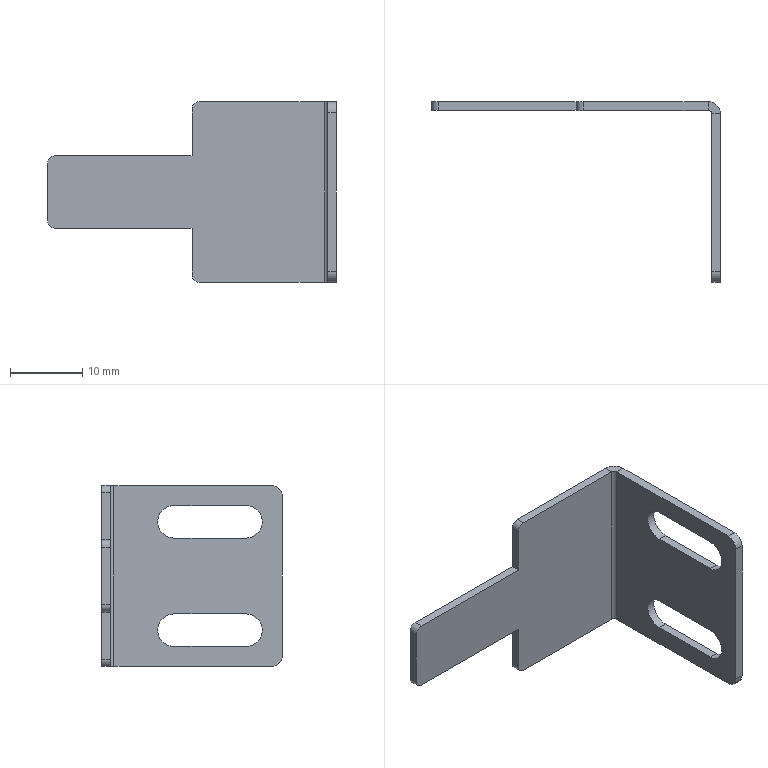Part | SolidWorks | features Fillet 2, FlatPattern 1, HoleWzd 1, ICE 1, SMBaseFlange 1, SheetMetal 1 | 1 solid | 32 faces | box 40 x 25 x 25 mm | volume 1391 mm3 | plane 20 | cylinder 12 | commonest cylinder face diameters 2 x4 4.5 x4 3 x2 1 x1 3.4 x1
STEP:
#1=CARTESIAN_POINT('',(0.,-10.,-5.25));
#2=VERTEX_POINT('',#1);
#3=CARTESIAN_POINT('',(0.,-10.,-9.75));
#4=VERTEX_POINT('',#3);
#5=CARTESIAN_POINT('',(0.,-10.,-7.5));
#6=DIRECTION('',(-1.,0.,0.));
#7=DIRECTION('',(0.,0.,1.));
#8=AXIS2_PLACEMENT_3D('',#5,#6,#7);
#9=CIRCLE('',#8,2.25);
#10=EDGE_CURVE('',#2,#4,#9,.T.);
#11=ORIENTED_EDGE('',*,*,#10,.T.);
#12=CARTESIAN_POINT('',(0.,-20.,-9.75));
#13=VERTEX_POINT('',#12);
#14=CARTESIAN_POINT('',(0.,-20.,-9.75));
#15=DIRECTION('',(0.,1.,0.));
#16=VECTOR('',#15,1000.);
#17=LINE('',#14,#16);
#18=EDGE_CURVE('',#13,#4,#17,.T.);
#19=ORIENTED_EDGE('',*,*,#18,.F.);
#20=CARTESIAN_POINT('',(0.,-20.,-5.25));
#21=VERTEX_POINT('',#20);
#22=CARTESIAN_POINT('',(0.,-20.,-7.5));
#23=DIRECTION('',(-1.,0.,0.));
#24=DIRECTION('',(0.,0.,1.));
#25=AXIS2_PLACEMENT_3D('',#22,#23,#24);
#26=CIRCLE('',#25,2.25);
#27=EDGE_CURVE('',#13,#21,#26,.T.);
#28=ORIENTED_EDGE('',*,*,#27,.T.);
#29=CARTESIAN_POINT('',(0.,-20.,-5.25));
#30=DIRECTION('',(0.,1.,0.));
#31=VECTOR('',#30,1000.);
#32=LINE('',#29,#31);
#33=EDGE_CURVE('',#21,#2,#32,.T.);
#34=ORIENTED_EDGE('',*,*,#33,.T.);
#35=EDGE_LOOP('',(#11,#19,#28,#34));
#36=FACE_BOUND('',#35,.T.);
#37=CARTESIAN_POINT('',(0.,-25.,11.));
#38=VERTEX_POINT('',#37);
#39=CARTESIAN_POINT('',(0.,-25.,-11.));
#40=VERTEX_POINT('',#39);
#41=CARTESIAN_POINT('',(0.,-25.,12.5));
#42=DIRECTION('',(0.,0.,-1.));
#43=VECTOR('',#42,1000.);
#44=LINE('',#41,#43);
#45=EDGE_CURVE('',#38,#40,#44,.T.);
#46=ORIENTED_EDGE('',*,*,#45,.T.);
#47=CARTESIAN_POINT('',(0.,-23.5,-12.5));
#48=VERTEX_POINT('',#47);
#49=CARTESIAN_POINT('',(0.,-23.5,-11.));
#50=DIRECTION('',(1.,0.,0.));
#51=DIRECTION('',(0.,0.,-1.));
#52=AXIS2_PLACEMENT_3D('',#49,#50,#51);
#53=CIRCLE('',#52,1.5);
#54=EDGE_CURVE('',#40,#48,#53,.T.);
#55=ORIENTED_EDGE('',*,*,#54,.T.);
#56=CARTESIAN_POINT('',(0.,-1.7,-12.5));
#57=VERTEX_POINT('',#56);
#58=CARTESIAN_POINT('',(0.,0.,-12.5));
#59=DIRECTION('',(0.,-1.,0.));
#60=VECTOR('',#59,1000.);
#61=LINE('',#58,#60);
#62=EDGE_CURVE('',#57,#48,#61,.T.);
#63=ORIENTED_EDGE('',*,*,#62,.F.);
#64=CARTESIAN_POINT('',(0.,-1.7,12.5));
#65=VERTEX_POINT('',#64);
#66=CARTESIAN_POINT('',(0.,-1.7,12.5));
#67=DIRECTION('',(0.,0.,-1.));
#68=VECTOR('',#67,1000.);
#69=LINE('',#66,#68);
#70=EDGE_CURVE('',#65,#57,#69,.T.);
#71=ORIENTED_EDGE('',*,*,#70,.F.);
#72=CARTESIAN_POINT('',(0.,-23.5,12.5));
#73=VERTEX_POINT('',#72);
#74=CARTESIAN_POINT('',(0.,0.,12.5));
#75=DIRECTION('',(0.,-1.,0.));
#76=VECTOR('',#75,1000.);
#77=LINE('',#74,#76);
#78=EDGE_CURVE('',#65,#73,#77,.T.);
#79=ORIENTED_EDGE('',*,*,#78,.T.);
#80=CARTESIAN_POINT('',(0.,-23.5,11.));
#81=DIRECTION('',(1.,0.,0.));
#82=DIRECTION('',(0.,0.,-1.));
#83=AXIS2_PLACEMENT_3D('',#80,#81,#82);
#84=CIRCLE('',#83,1.5);
#85=EDGE_CURVE('',#73,#38,#84,.T.);
#86=ORIENTED_EDGE('',*,*,#85,.T.);
#87=EDGE_LOOP('',(#46,#55,#63,#71,#79,#86));
#88=FACE_OUTER_BOUND('',#87,.T.);
#89=CARTESIAN_POINT('',(0.,-20.,5.25));
#90=VERTEX_POINT('',#89);
#91=CARTESIAN_POINT('',(0.,-20.,9.75));
#92=VERTEX_POINT('',#91);
#93=CARTESIAN_POINT('',(0.,-20.,7.5));
#94=DIRECTION('',(-1.,0.,0.));
#95=DIRECTION('',(0.,0.,1.));
#96=AXIS2_PLACEMENT_3D('',#93,#94,#95);
#97=CIRCLE('',#96,2.25);
#98=EDGE_CURVE('',#90,#92,#97,.T.);
#99=ORIENTED_EDGE('',*,*,#98,.T.);
#100=CARTESIAN_POINT('',(0.,-10.,9.75));
#101=VERTEX_POINT('',#100);
#102=CARTESIAN_POINT('',(0.,-20.,9.75));
#103=DIRECTION('',(0.,1.,0.));
#104=VECTOR('',#103,1000.);
#105=LINE('',#102,#104);
#106=EDGE_CURVE('',#92,#101,#105,.T.);
#107=ORIENTED_EDGE('',*,*,#106,.T.);
#108=CARTESIAN_POINT('',(0.,-10.,5.25));
#109=VERTEX_POINT('',#108);
#110=CARTESIAN_POINT('',(0.,-10.,7.5));
#111=DIRECTION('',(-1.,0.,0.));
#112=DIRECTION('',(0.,0.,1.));
#113=AXIS2_PLACEMENT_3D('',#110,#111,#112);
#114=CIRCLE('',#113,2.25);
#115=EDGE_CURVE('',#101,#109,#114,.T.);
#116=ORIENTED_EDGE('',*,*,#115,.T.);
#117=CARTESIAN_POINT('',(0.,-20.,5.25));
#118=DIRECTION('',(0.,1.,0.));
#119=VECTOR('',#118,1000.);
#120=LINE('',#117,#119);
#121=EDGE_CURVE('',#90,#109,#120,.T.);
#122=ORIENTED_EDGE('',*,*,#121,.F.);
#123=EDGE_LOOP('',(#99,#107,#116,#122));
#124=FACE_BOUND('',#123,.T.);
#125=CARTESIAN_POINT('',(0.,0.,12.5));
#126=DIRECTION('',(1.,0.,0.));
#127=DIRECTION('',(0.,0.,-1.));
#128=AXIS2_PLACEMENT_3D('',#125,#126,#127);
#129=PLANE('',#128);
#130=ADVANCED_FACE('',(#36,#88,#124),#129,.T.);
#131=CARTESIAN_POINT('',(-1.2,-1.7,12.5));
#132=VERTEX_POINT('',#131);
#133=CARTESIAN_POINT('',(0.,-1.7,12.5));
#134=DIRECTION('',(-1.,0.,0.));
#135=VECTOR('',#134,1000.);
#136=LINE('',#133,#135);
#137=EDGE_CURVE('',#65,#132,#136,.T.);
#138=ORIENTED_EDGE('',*,*,#137,.F.);
#139=CARTESIAN_POINT('',(-1.7,0.,12.5));
#140=VERTEX_POINT('',#139);
#141=CARTESIAN_POINT('',(-1.7,-1.7,12.5));
#142=DIRECTION('',(0.,0.,-1.));
#143=DIRECTION('',(1.,0.,0.));
#144=AXIS2_PLACEMENT_3D('',#141,#142,#143);
#145=CIRCLE('',#144,1.7);
#146=EDGE_CURVE('',#140,#65,#145,.T.);
#147=ORIENTED_EDGE('',*,*,#146,.F.);
#148=CARTESIAN_POINT('',(-1.7,-1.2,12.5));
#149=VERTEX_POINT('',#148);
#150=CARTESIAN_POINT('',(-1.7,-1.2,12.5));
#151=DIRECTION('',(0.,1.,0.));
#152=VECTOR('',#151,1000.);
#153=LINE('',#150,#152);
#154=EDGE_CURVE('',#149,#140,#153,.T.);
#155=ORIENTED_EDGE('',*,*,#154,.F.);
#156=CARTESIAN_POINT('',(-1.7,-1.7,12.5));
#157=DIRECTION('',(0.,0.,-1.));
#158=DIRECTION('',(1.,0.,0.));
#159=AXIS2_PLACEMENT_3D('',#156,#157,#158);
#160=CIRCLE('',#159,0.5);
#161=EDGE_CURVE('',#149,#132,#160,.T.);
#162=ORIENTED_EDGE('',*,*,#161,.T.);
#163=EDGE_LOOP('',(#138,#147,#155,#162));
#164=FACE_OUTER_BOUND('',#163,.T.);
#165=CARTESIAN_POINT('',(0.,-1.7,12.5));
#166=DIRECTION('',(0.,0.,1.));
#167=DIRECTION('',(1.,0.,0.));
#168=AXIS2_PLACEMENT_3D('',#165,#166,#167);
#169=PLANE('',#168);
#170=ADVANCED_FACE('',(#164),#169,.T.);
#171=CARTESIAN_POINT('',(-1.2,-23.5,12.5));
#172=VERTEX_POINT('',#171);
#173=CARTESIAN_POINT('',(-1.2,0.,12.5));
#174=DIRECTION('',(0.,-1.,0.));
#175=VECTOR('',#174,1000.);
#176=LINE('',#173,#175);
#177=EDGE_CURVE('',#132,#172,#176,.T.);
#178=ORIENTED_EDGE('',*,*,#177,.T.);
#179=CARTESIAN_POINT('',(-1.7,-23.5,12.5));
#180=DIRECTION('',(1.,0.,0.));
#181=VECTOR('',#180,1000.);
#182=LINE('',#179,#181);
#183=EDGE_CURVE('',#172,#73,#182,.T.);
#184=ORIENTED_EDGE('',*,*,#183,.T.);
#185=ORIENTED_EDGE('',*,*,#78,.F.);
#186=ORIENTED_EDGE('',*,*,#137,.T.);
#187=EDGE_LOOP('',(#178,#184,#185,#186));
#188=FACE_OUTER_BOUND('',#187,.T.);
#189=CARTESIAN_POINT('',(-1.7,-1.2,12.5));
#190=DIRECTION('',(0.,0.,1.));
#191=DIRECTION('',(1.,0.,0.));
#192=AXIS2_PLACEMENT_3D('',#189,#190,#191);
#193=PLANE('',#192);
#194=ADVANCED_FACE('',(#188),#193,.T.);
#195=CARTESIAN_POINT('',(-1.7,0.,-12.5));
#196=VERTEX_POINT('',#195);
#197=CARTESIAN_POINT('',(-1.7,-1.2,-12.5));
#198=VERTEX_POINT('',#197);
#199=CARTESIAN_POINT('',(-1.7,0.,-12.5));
#200=DIRECTION('',(0.,-1.,0.));
#201=VECTOR('',#200,1000.);
#202=LINE('',#199,#201);
#203=EDGE_CURVE('',#196,#198,#202,.T.);
#204=ORIENTED_EDGE('',*,*,#203,.F.);
#205=CARTESIAN_POINT('',(-1.7,-1.7,-12.5));
#206=DIRECTION('',(0.,0.,-1.));
#207=DIRECTION('',(1.,0.,0.));
#208=AXIS2_PLACEMENT_3D('',#205,#206,#207);
#209=CIRCLE('',#208,1.7);
#210=EDGE_CURVE('',#196,#57,#209,.T.);
#211=ORIENTED_EDGE('',*,*,#210,.T.);
#212=CARTESIAN_POINT('',(-1.2,-1.7,-12.5));
#213=VERTEX_POINT('',#212);
#214=CARTESIAN_POINT('',(-1.2,-1.7,-12.5));
#215=DIRECTION('',(1.,0.,0.));
#216=VECTOR('',#215,1000.);
#217=LINE('',#214,#216);
#218=EDGE_CURVE('',#213,#57,#217,.T.);
#219=ORIENTED_EDGE('',*,*,#218,.F.);
#220=CARTESIAN_POINT('',(-1.7,-1.7,-12.5));
#221=DIRECTION('',(0.,0.,-1.));
#222=DIRECTION('',(1.,0.,0.));
#223=AXIS2_PLACEMENT_3D('',#220,#221,#222);
#224=CIRCLE('',#223,0.5);
#225=EDGE_CURVE('',#198,#213,#224,.T.);
#226=ORIENTED_EDGE('',*,*,#225,.F.);
#227=EDGE_LOOP('',(#204,#211,#219,#226));
#228=FACE_OUTER_BOUND('',#227,.T.);
#229=CARTESIAN_POINT('',(-1.7,0.,-12.5));
#230=DIRECTION('',(0.,0.,-1.));
#231=DIRECTION('',(-1.,0.,0.));
#232=AXIS2_PLACEMENT_3D('',#229,#230,#231);
#233=PLANE('',#232);
#234=ADVANCED_FACE('',(#228),#233,.T.);
#235=CARTESIAN_POINT('',(-19.,-1.2,-12.5));
#236=VERTEX_POINT('',#235);
#237=CARTESIAN_POINT('',(-40.,-1.2,-12.5));
#238=DIRECTION('',(1.,0.,0.));
#239=VECTOR('',#238,1000.);
#240=LINE('',#237,#239);
#241=EDGE_CURVE('',#236,#198,#240,.T.);
#242=ORIENTED_EDGE('',*,*,#241,.F.);
#243=CARTESIAN_POINT('',(-19.,0.,-12.5));
#244=VERTEX_POINT('',#243);
#245=CARTESIAN_POINT('',(-19.,0.,-12.5));
#246=DIRECTION('',(0.,1.,0.));
#247=VECTOR('',#246,1000.);
#248=LINE('',#245,#247);
#249=EDGE_CURVE('',#236,#244,#248,.T.);
#250=ORIENTED_EDGE('',*,*,#249,.T.);
#251=CARTESIAN_POINT('',(-40.,0.,-12.5));
#252=DIRECTION('',(1.,0.,0.));
#253=VECTOR('',#252,1000.);
#254=LINE('',#251,#253);
#255=EDGE_CURVE('',#244,#196,#254,.T.);
#256=ORIENTED_EDGE('',*,*,#255,.T.);
#257=ORIENTED_EDGE('',*,*,#203,.T.);
#258=EDGE_LOOP('',(#242,#250,#256,#257));
#259=FACE_OUTER_BOUND('',#258,.T.);
#260=CARTESIAN_POINT('',(-1.2,-1.7,-12.5));
#261=DIRECTION('',(0.,0.,-1.));
#262=DIRECTION('',(-1.,0.,0.));
#263=AXIS2_PLACEMENT_3D('',#260,#261,#262);
#264=PLANE('',#263);
#265=ADVANCED_FACE('',(#259),#264,.T.);
#266=CARTESIAN_POINT('',(-1.2,-20.,5.25));
#267=VERTEX_POINT('',#266);
#268=CARTESIAN_POINT('',(-1.2,-20.,9.75));
#269=VERTEX_POINT('',#268);
#270=CARTESIAN_POINT('',(-1.2,-20.,7.5));
#271=DIRECTION('',(-1.,0.,0.));
#272=DIRECTION('',(0.,0.,1.));
#273=AXIS2_PLACEMENT_3D('',#270,#271,#272);
#274=CIRCLE('',#273,2.25);
#275=EDGE_CURVE('',#267,#269,#274,.T.);
#276=ORIENTED_EDGE('',*,*,#275,.F.);
#277=CARTESIAN_POINT('',(-1.2,-10.,5.25));
#278=VERTEX_POINT('',#277);
#279=CARTESIAN_POINT('',(-1.2,-20.,5.25));
#280=DIRECTION('',(0.,1.,0.));
#281=VECTOR('',#280,1000.);
#282=LINE('',#279,#281);
#283=EDGE_CURVE('',#267,#278,#282,.T.);
#284=ORIENTED_EDGE('',*,*,#283,.T.);
#285=CARTESIAN_POINT('',(-1.2,-10.,9.75));
#286=VERTEX_POINT('',#285);
#287=CARTESIAN_POINT('',(-1.2,-10.,7.5));
#288=DIRECTION('',(-1.,0.,0.));
#289=DIRECTION('',(0.,0.,1.));
#290=AXIS2_PLACEMENT_3D('',#287,#288,#289);
#291=CIRCLE('',#290,2.25);
#292=EDGE_CURVE('',#286,#278,#291,.T.);
#293=ORIENTED_EDGE('',*,*,#292,.F.);
#294=CARTESIAN_POINT('',(-1.2,-20.,9.75));
#295=DIRECTION('',(0.,1.,0.));
#296=VECTOR('',#295,1000.);
#297=LINE('',#294,#296);
#298=EDGE_CURVE('',#269,#286,#297,.T.);
#299=ORIENTED_EDGE('',*,*,#298,.F.);
#300=EDGE_LOOP('',(#276,#284,#293,#299));
#301=FACE_BOUND('',#300,.T.);
#302=CARTESIAN_POINT('',(-1.2,-20.,-9.75));
#303=VERTEX_POINT('',#302);
#304=CARTESIAN_POINT('',(-1.2,-10.,-9.75));
#305=VERTEX_POINT('',#304);
#306=CARTESIAN_POINT('',(-1.2,-20.,-9.75));
#307=DIRECTION('',(0.,1.,0.));
#308=VECTOR('',#307,1000.);
#309=LINE('',#306,#308);
#310=EDGE_CURVE('',#303,#305,#309,.T.);
#311=ORIENTED_EDGE('',*,*,#310,.T.);
#312=CARTESIAN_POINT('',(-1.2,-10.,-5.25));
#313=VERTEX_POINT('',#312);
#314=CARTESIAN_POINT('',(-1.2,-10.,-7.5));
#315=DIRECTION('',(-1.,0.,0.));
#316=DIRECTION('',(0.,0.,1.));
#317=AXIS2_PLACEMENT_3D('',#314,#315,#316);
#318=CIRCLE('',#317,2.25);
#319=EDGE_CURVE('',#313,#305,#318,.T.);
#320=ORIENTED_EDGE('',*,*,#319,.F.);
#321=CARTESIAN_POINT('',(-1.2,-20.,-5.25));
#322=VERTEX_POINT('',#321);
#323=CARTESIAN_POINT('',(-1.2,-20.,-5.25));
#324=DIRECTION('',(0.,1.,0.));
#325=VECTOR('',#324,1000.);
#326=LINE('',#323,#325);
#327=EDGE_CURVE('',#322,#313,#326,.T.);
#328=ORIENTED_EDGE('',*,*,#327,.F.);
#329=CARTESIAN_POINT('',(-1.2,-20.,-7.5));
#330=DIRECTION('',(-1.,0.,0.));
#331=DIRECTION('',(0.,0.,1.));
#332=AXIS2_PLACEMENT_3D('',#329,#330,#331);
#333=CIRCLE('',#332,2.25);
#334=EDGE_CURVE('',#303,#322,#333,.T.);
#335=ORIENTED_EDGE('',*,*,#334,.F.);
#336=EDGE_LOOP('',(#311,#320,#328,#335));
#337=FACE_BOUND('',#336,.T.);
#338=CARTESIAN_POINT('',(-1.2,-23.5,-12.5));
#339=VERTEX_POINT('',#338);
#340=CARTESIAN_POINT('',(-1.2,0.,-12.5));
#341=DIRECTION('',(0.,-1.,0.));
#342=VECTOR('',#341,1000.);
#343=LINE('',#340,#342);
#344=EDGE_CURVE('',#213,#339,#343,.T.);
#345=ORIENTED_EDGE('',*,*,#344,.T.);
#346=CARTESIAN_POINT('',(-1.2,-25.,-11.));
#347=VERTEX_POINT('',#346);
#348=CARTESIAN_POINT('',(-1.2,-23.5,-11.));
#349=DIRECTION('',(-1.,0.,0.));
#350=DIRECTION('',(0.,0.,-1.));
#351=AXIS2_PLACEMENT_3D('',#348,#349,#350);
#352=CIRCLE('',#351,1.5);
#353=EDGE_CURVE('',#339,#347,#352,.T.);
#354=ORIENTED_EDGE('',*,*,#353,.T.);
#355=CARTESIAN_POINT('',(-1.2,-25.,11.));
#356=VERTEX_POINT('',#355);
#357=CARTESIAN_POINT('',(-1.2,-25.,12.5));
#358=DIRECTION('',(0.,0.,-1.));
#359=VECTOR('',#358,1000.);
#360=LINE('',#357,#359);
#361=EDGE_CURVE('',#356,#347,#360,.T.);
#362=ORIENTED_EDGE('',*,*,#361,.F.);
#363=CARTESIAN_POINT('',(-1.2,-23.5,11.));
#364=DIRECTION('',(-1.,0.,0.));
#365=DIRECTION('',(0.,0.,-1.));
#366=AXIS2_PLACEMENT_3D('',#363,#364,#365);
#367=CIRCLE('',#366,1.5);
#368=EDGE_CURVE('',#356,#172,#367,.T.);
#369=ORIENTED_EDGE('',*,*,#368,.T.);
#370=ORIENTED_EDGE('',*,*,#177,.F.);
#371=CARTESIAN_POINT('',(-1.2,-1.7,12.5));
#372=DIRECTION('',(0.,0.,-1.));
#373=VECTOR('',#372,1000.);
#374=LINE('',#371,#373);
#375=EDGE_CURVE('',#132,#213,#374,.T.);
#376=ORIENTED_EDGE('',*,*,#375,.T.);
#377=EDGE_LOOP('',(#345,#354,#362,#369,#370,#376));
#378=FACE_OUTER_BOUND('',#377,.T.);
#379=CARTESIAN_POINT('',(-1.2,0.,12.5));
#380=DIRECTION('',(1.,0.,0.));
#381=DIRECTION('',(0.,0.,-1.));
#382=AXIS2_PLACEMENT_3D('',#379,#380,#381);
#383=PLANE('',#382);
#384=ADVANCED_FACE('',(#301,#337,#378),#383,.F.);
#385=ORIENTED_EDGE('',*,*,#361,.T.);
#386=CARTESIAN_POINT('',(0.,-25.,-11.));
#387=DIRECTION('',(1.,0.,0.));
#388=VECTOR('',#387,1000.);
#389=LINE('',#386,#388);
#390=EDGE_CURVE('',#347,#40,#389,.T.);
#391=ORIENTED_EDGE('',*,*,#390,.T.);
#392=ORIENTED_EDGE('',*,*,#45,.F.);
#393=CARTESIAN_POINT('',(0.,-25.,11.));
#394=DIRECTION('',(-1.,0.,0.));
#395=VECTOR('',#394,1000.);
#396=LINE('',#393,#395);
#397=EDGE_CURVE('',#38,#356,#396,.T.);
#398=ORIENTED_EDGE('',*,*,#397,.T.);
#399=EDGE_LOOP('',(#385,#391,#392,#398));
#400=FACE_OUTER_BOUND('',#399,.T.);
#401=CARTESIAN_POINT('',(0.,-25.,12.5));
#402=DIRECTION('',(0.,-1.,0.));
#403=DIRECTION('',(0.,0.,-1.));
#404=AXIS2_PLACEMENT_3D('',#401,#402,#403);
#405=PLANE('',#404);
#406=ADVANCED_FACE('',(#400),#405,.T.);
#407=ORIENTED_EDGE('',*,*,#210,.F.);
#408=CARTESIAN_POINT('',(-1.7,0.,12.5));
#409=DIRECTION('',(0.,0.,-1.));
#410=VECTOR('',#409,1000.);
#411=LINE('',#408,#410);
#412=EDGE_CURVE('',#140,#196,#411,.T.);
#413=ORIENTED_EDGE('',*,*,#412,.F.);
#414=ORIENTED_EDGE('',*,*,#146,.T.);
#415=ORIENTED_EDGE('',*,*,#70,.T.);
#416=EDGE_LOOP('',(#407,#413,#414,#415));
#417=FACE_OUTER_BOUND('',#416,.T.);
#418=CARTESIAN_POINT('',(-1.7,-1.7,12.5));
#419=DIRECTION('',(0.,0.,-1.));
#420=DIRECTION('',(-1.,0.,0.));
#421=AXIS2_PLACEMENT_3D('',#418,#419,#420);
#422=CYLINDRICAL_SURFACE('',#421,1.7);
#423=ADVANCED_FACE('',(#417),#422,.T.);
#424=CARTESIAN_POINT('',(-20.,0.,11.5));
#425=VERTEX_POINT('',#424);
#426=CARTESIAN_POINT('',(-20.,0.,5.));
#427=VERTEX_POINT('',#426);
#428=CARTESIAN_POINT('',(-20.,0.,12.5));
#429=DIRECTION('',(0.,0.,-1.));
#430=VECTOR('',#429,1000.);
#431=LINE('',#428,#430);
#432=EDGE_CURVE('',#425,#427,#431,.T.);
#433=ORIENTED_EDGE('',*,*,#432,.F.);
#434=CARTESIAN_POINT('',(-19.,0.,12.5));
#435=VERTEX_POINT('',#434);
#436=CARTESIAN_POINT('',(-19.,0.,11.5));
#437=DIRECTION('',(0.,1.,0.));
#438=DIRECTION('',(0.,0.,1.));
#439=AXIS2_PLACEMENT_3D('',#436,#437,#438);
#440=CIRCLE('',#439,1.);
#441=EDGE_CURVE('',#425,#435,#440,.T.);
#442=ORIENTED_EDGE('',*,*,#441,.T.);
#443=CARTESIAN_POINT('',(-40.,0.,12.5));
#444=DIRECTION('',(1.,0.,0.));
#445=VECTOR('',#444,1000.);
#446=LINE('',#443,#445);
#447=EDGE_CURVE('',#435,#140,#446,.T.);
#448=ORIENTED_EDGE('',*,*,#447,.T.);
#449=ORIENTED_EDGE('',*,*,#412,.T.);
#450=ORIENTED_EDGE('',*,*,#255,.F.);
#451=CARTESIAN_POINT('',(-20.,0.,-11.5));
#452=VERTEX_POINT('',#451);
#453=CARTESIAN_POINT('',(-19.,0.,-11.5));
#454=DIRECTION('',(0.,1.,0.));
#455=DIRECTION('',(0.,0.,1.));
#456=AXIS2_PLACEMENT_3D('',#453,#454,#455);
#457=CIRCLE('',#456,1.);
#458=EDGE_CURVE('',#244,#452,#457,.T.);
#459=ORIENTED_EDGE('',*,*,#458,.T.);
#460=CARTESIAN_POINT('',(-20.,0.,-5.));
#461=VERTEX_POINT('',#460);
#462=CARTESIAN_POINT('',(-20.,0.,-12.5));
#463=DIRECTION('',(0.,0.,-1.));
#464=VECTOR('',#463,1000.);
#465=LINE('',#462,#464);
#466=EDGE_CURVE('',#461,#452,#465,.T.);
#467=ORIENTED_EDGE('',*,*,#466,.F.);
#468=CARTESIAN_POINT('',(-39.,0.,-5.));
#469=VERTEX_POINT('',#468);
#470=CARTESIAN_POINT('',(-40.,0.,-5.));
#471=DIRECTION('',(1.,0.,0.));
#472=VECTOR('',#471,1000.);
#473=LINE('',#470,#472);
#474=EDGE_CURVE('',#469,#461,#473,.T.);
#475=ORIENTED_EDGE('',*,*,#474,.F.);
#476=CARTESIAN_POINT('',(-40.,0.,-4.));
#477=VERTEX_POINT('',#476);
#478=CARTESIAN_POINT('',(-39.,0.,-4.));
#479=DIRECTION('',(0.,1.,0.));
#480=DIRECTION('',(0.,0.,1.));
#481=AXIS2_PLACEMENT_3D('',#478,#479,#480);
#482=CIRCLE('',#481,1.);
#483=EDGE_CURVE('',#469,#477,#482,.T.);
#484=ORIENTED_EDGE('',*,*,#483,.T.);
#485=CARTESIAN_POINT('',(-40.,0.,4.));
#486=VERTEX_POINT('',#485);
#487=CARTESIAN_POINT('',(-40.,0.,12.5));
#488=DIRECTION('',(0.,0.,-1.));
#489=VECTOR('',#488,1000.);
#490=LINE('',#487,#489);
#491=EDGE_CURVE('',#486,#477,#490,.T.);
#492=ORIENTED_EDGE('',*,*,#491,.F.);
#493=CARTESIAN_POINT('',(-39.,0.,5.));
#494=VERTEX_POINT('',#493);
#495=CARTESIAN_POINT('',(-39.,0.,4.));
#496=DIRECTION('',(0.,1.,0.));
#497=DIRECTION('',(0.,0.,1.));
#498=AXIS2_PLACEMENT_3D('',#495,#496,#497);
#499=CIRCLE('',#498,1.);
#500=EDGE_CURVE('',#486,#494,#499,.T.);
#501=ORIENTED_EDGE('',*,*,#500,.T.);
#502=CARTESIAN_POINT('',(-40.,0.,5.));
#503=DIRECTION('',(-1.,0.,0.));
#504=VECTOR('',#503,1000.);
#505=LINE('',#502,#504);
#506=EDGE_CURVE('',#427,#494,#505,.T.);
#507=ORIENTED_EDGE('',*,*,#506,.F.);
#508=EDGE_LOOP('',(#433,#442,#448,#449,#450,#459,#467,#475,#484,#492,#501,#507));
#509=FACE_OUTER_BOUND('',#508,.T.);
#510=CARTESIAN_POINT('',(-40.,0.,12.5));
#511=DIRECTION('',(0.,1.,0.));
#512=DIRECTION('',(0.,0.,1.));
#513=AXIS2_PLACEMENT_3D('',#510,#511,#512);
#514=PLANE('',#513);
#515=ADVANCED_FACE('',(#509),#514,.T.);
#516=ORIENTED_EDGE('',*,*,#491,.T.);
#517=CARTESIAN_POINT('',(-40.,-1.2,-4.));
#518=VERTEX_POINT('',#517);
#519=CARTESIAN_POINT('',(-40.,-1.2,-4.));
#520=DIRECTION('',(0.,-1.,0.));
#521=VECTOR('',#520,1000.);
#522=LINE('',#519,#521);
#523=EDGE_CURVE('',#477,#518,#522,.T.);
#524=ORIENTED_EDGE('',*,*,#523,.T.);
#525=CARTESIAN_POINT('',(-40.,-1.2,4.));
#526=VERTEX_POINT('',#525);
#527=CARTESIAN_POINT('',(-40.,-1.2,12.5));
#528=DIRECTION('',(0.,0.,-1.));
#529=VECTOR('',#528,1000.);
#530=LINE('',#527,#529);
#531=EDGE_CURVE('',#526,#518,#530,.T.);
#532=ORIENTED_EDGE('',*,*,#531,.F.);
#533=CARTESIAN_POINT('',(-40.,0.,4.));
#534=DIRECTION('',(0.,1.,0.));
#535=VECTOR('',#534,1000.);
#536=LINE('',#533,#535);
#537=EDGE_CURVE('',#526,#486,#536,.T.);
#538=ORIENTED_EDGE('',*,*,#537,.T.);
#539=EDGE_LOOP('',(#516,#524,#532,#538));
#540=FACE_OUTER_BOUND('',#539,.T.);
#541=CARTESIAN_POINT('',(-40.,-1.2,12.5));
#542=DIRECTION('',(-1.,0.,0.));
#543=DIRECTION('',(0.,0.,1.));
#544=AXIS2_PLACEMENT_3D('',#541,#542,#543);
#545=PLANE('',#544);
#546=ADVANCED_FACE('',(#540),#545,.T.);
#547=CARTESIAN_POINT('',(-19.,-1.2,12.5));
#548=VERTEX_POINT('',#547);
#549=CARTESIAN_POINT('',(-40.,-1.2,12.5));
#550=DIRECTION('',(1.,0.,0.));
#551=VECTOR('',#550,1000.);
#552=LINE('',#549,#551);
#553=EDGE_CURVE('',#548,#149,#552,.T.);
#554=ORIENTED_EDGE('',*,*,#553,.F.);
#555=CARTESIAN_POINT('',(-20.,-1.2,11.5));
#556=VERTEX_POINT('',#555);
#557=CARTESIAN_POINT('',(-19.,-1.2,11.5));
#558=DIRECTION('',(0.,-1.,0.));
#559=DIRECTION('',(0.,0.,1.));
#560=AXIS2_PLACEMENT_3D('',#557,#558,#559);
#561=CIRCLE('',#560,1.);
#562=EDGE_CURVE('',#548,#556,#561,.T.);
#563=ORIENTED_EDGE('',*,*,#562,.T.);
#564=CARTESIAN_POINT('',(-20.,-1.2,5.));
#565=VERTEX_POINT('',#564);
#566=CARTESIAN_POINT('',(-20.,-1.2,12.5));
#567=DIRECTION('',(0.,0.,1.));
#568=VECTOR('',#567,1000.);
#569=LINE('',#566,#568);
#570=EDGE_CURVE('',#565,#556,#569,.T.);
#571=ORIENTED_EDGE('',*,*,#570,.F.);
#572=CARTESIAN_POINT('',(-39.,-1.2,5.));
#573=VERTEX_POINT('',#572);
#574=CARTESIAN_POINT('',(-40.,-1.2,5.));
#575=DIRECTION('',(1.,0.,0.));
#576=VECTOR('',#575,1000.);
#577=LINE('',#574,#576);
#578=EDGE_CURVE('',#573,#565,#577,.T.);
#579=ORIENTED_EDGE('',*,*,#578,.F.);
#580=CARTESIAN_POINT('',(-39.,-1.2,4.));
#581=DIRECTION('',(0.,-1.,0.));
#582=DIRECTION('',(0.,0.,1.));
#583=AXIS2_PLACEMENT_3D('',#580,#581,#582);
#584=CIRCLE('',#583,1.);
#585=EDGE_CURVE('',#573,#526,#584,.T.);
#586=ORIENTED_EDGE('',*,*,#585,.T.);
#587=ORIENTED_EDGE('',*,*,#531,.T.);
#588=CARTESIAN_POINT('',(-39.,-1.2,-5.));
#589=VERTEX_POINT('',#588);
#590=CARTESIAN_POINT('',(-39.,-1.2,-4.));
#591=DIRECTION('',(0.,-1.,0.));
#592=DIRECTION('',(0.,0.,1.));
#593=AXIS2_PLACEMENT_3D('',#590,#591,#592);
#594=CIRCLE('',#593,1.);
#595=EDGE_CURVE('',#518,#589,#594,.T.);
#596=ORIENTED_EDGE('',*,*,#595,.T.);
#597=CARTESIAN_POINT('',(-20.,-1.2,-5.));
#598=VERTEX_POINT('',#597);
#599=CARTESIAN_POINT('',(-40.,-1.2,-5.));
#600=DIRECTION('',(-1.,0.,0.));
#601=VECTOR('',#600,1000.);
#602=LINE('',#599,#601);
#603=EDGE_CURVE('',#598,#589,#602,.T.);
#604=ORIENTED_EDGE('',*,*,#603,.F.);
#605=CARTESIAN_POINT('',(-20.,-1.2,-11.5));
#606=VERTEX_POINT('',#605);
#607=CARTESIAN_POINT('',(-20.,-1.2,-12.5));
#608=DIRECTION('',(0.,0.,1.));
#609=VECTOR('',#608,1000.);
#610=LINE('',#607,#609);
#611=EDGE_CURVE('',#606,#598,#610,.T.);
#612=ORIENTED_EDGE('',*,*,#611,.F.);
#613=CARTESIAN_POINT('',(-19.,-1.2,-11.5));
#614=DIRECTION('',(0.,-1.,0.));
#615=DIRECTION('',(0.,0.,1.));
#616=AXIS2_PLACEMENT_3D('',#613,#614,#615);
#617=CIRCLE('',#616,1.);
#618=EDGE_CURVE('',#606,#236,#617,.T.);
#619=ORIENTED_EDGE('',*,*,#618,.T.);
#620=ORIENTED_EDGE('',*,*,#241,.T.);
#621=CARTESIAN_POINT('',(-1.7,-1.2,12.5));
#622=DIRECTION('',(0.,0.,-1.));
#623=VECTOR('',#622,1000.);
#624=LINE('',#621,#623);
#625=EDGE_CURVE('',#149,#198,#624,.T.);
#626=ORIENTED_EDGE('',*,*,#625,.F.);
#627=EDGE_LOOP('',(#554,#563,#571,#579,#586,#587,#596,#604,#612,#619,#620,#626));
#628=FACE_OUTER_BOUND('',#627,.T.);
#629=CARTESIAN_POINT('',(-40.,-1.2,12.5));
#630=DIRECTION('',(0.,1.,0.));
#631=DIRECTION('',(0.,0.,1.));
#632=AXIS2_PLACEMENT_3D('',#629,#630,#631);
#633=PLANE('',#632);
#634=ADVANCED_FACE('',(#628),#633,.F.);
#635=ORIENTED_EDGE('',*,*,#225,.T.);
#636=ORIENTED_EDGE('',*,*,#375,.F.);
#637=ORIENTED_EDGE('',*,*,#161,.F.);
#638=ORIENTED_EDGE('',*,*,#625,.T.);
#639=EDGE_LOOP('',(#635,#636,#637,#638));
#640=FACE_OUTER_BOUND('',#639,.T.);
#641=CARTESIAN_POINT('',(-1.7,-1.7,12.5));
#642=DIRECTION('',(0.,0.,-1.));
#643=DIRECTION('',(-1.,0.,0.));
#644=AXIS2_PLACEMENT_3D('',#641,#642,#643);
#645=CYLINDRICAL_SURFACE('',#644,0.5);
#646=ADVANCED_FACE('',(#640),#645,.F.);
#647=ORIENTED_EDGE('',*,*,#447,.F.);
#648=CARTESIAN_POINT('',(-19.,-1.2,12.5));
#649=DIRECTION('',(0.,-1.,0.));
#650=VECTOR('',#649,1000.);
#651=LINE('',#648,#650);
#652=EDGE_CURVE('',#435,#548,#651,.T.);
#653=ORIENTED_EDGE('',*,*,#652,.T.);
#654=ORIENTED_EDGE('',*,*,#553,.T.);
#655=ORIENTED_EDGE('',*,*,#154,.T.);
#656=EDGE_LOOP('',(#647,#653,#654,#655));
#657=FACE_OUTER_BOUND('',#656,.T.);
#658=CARTESIAN_POINT('',(-1.7,-1.7,12.5));
#659=DIRECTION('',(0.,0.,1.));
#660=DIRECTION('',(1.,0.,0.));
#661=AXIS2_PLACEMENT_3D('',#658,#659,#660);
#662=PLANE('',#661);
#663=ADVANCED_FACE('',(#657),#662,.T.);
#664=ORIENTED_EDGE('',*,*,#62,.T.);
#665=CARTESIAN_POINT('',(-1.2,-23.5,-12.5));
#666=DIRECTION('',(-1.,0.,0.));
#667=VECTOR('',#666,1000.);
#668=LINE('',#665,#667);
#669=EDGE_CURVE('',#48,#339,#668,.T.);
#670=ORIENTED_EDGE('',*,*,#669,.T.);
#671=ORIENTED_EDGE('',*,*,#344,.F.);
#672=ORIENTED_EDGE('',*,*,#218,.T.);
#673=EDGE_LOOP('',(#664,#670,#671,#672));
#674=FACE_OUTER_BOUND('',#673,.T.);
#675=CARTESIAN_POINT('',(-1.7,-1.7,-12.5));
#676=DIRECTION('',(0.,0.,1.));
#677=DIRECTION('',(1.,0.,0.));
#678=AXIS2_PLACEMENT_3D('',#675,#676,#677);
#679=PLANE('',#678);
#680=ADVANCED_FACE('',(#674),#679,.F.);
#681=ORIENTED_EDGE('',*,*,#506,.T.);
#682=CARTESIAN_POINT('',(-39.,-1.2,5.));
#683=DIRECTION('',(0.,-1.,0.));
#684=VECTOR('',#683,1000.);
#685=LINE('',#682,#684);
#686=EDGE_CURVE('',#494,#573,#685,.T.);
#687=ORIENTED_EDGE('',*,*,#686,.T.);
#688=ORIENTED_EDGE('',*,*,#578,.T.);
#689=CARTESIAN_POINT('',(-20.,-22.56,5.));
#690=DIRECTION('',(0.,1.,0.));
#691=VECTOR('',#690,1000.);
#692=LINE('',#689,#691);
#693=EDGE_CURVE('',#565,#427,#692,.T.);
#694=ORIENTED_EDGE('',*,*,#693,.T.);
#695=EDGE_LOOP('',(#681,#687,#688,#694));
#696=FACE_OUTER_BOUND('',#695,.T.);
#697=CARTESIAN_POINT('',(-40.,-22.56,5.));
#698=DIRECTION('',(0.,0.,-1.));
#699=DIRECTION('',(-1.,0.,0.));
#700=AXIS2_PLACEMENT_3D('',#697,#698,#699);
#701=PLANE('',#700);
#702=ADVANCED_FACE('',(#696),#701,.F.);
#703=ORIENTED_EDGE('',*,*,#570,.T.);
#704=CARTESIAN_POINT('',(-20.,0.,11.5));
#705=DIRECTION('',(0.,1.,0.));
#706=VECTOR('',#705,1000.);
#707=LINE('',#704,#706);
#708=EDGE_CURVE('',#556,#425,#707,.T.);
#709=ORIENTED_EDGE('',*,*,#708,.T.);
#710=ORIENTED_EDGE('',*,*,#432,.T.);
#711=ORIENTED_EDGE('',*,*,#693,.F.);
#712=EDGE_LOOP('',(#703,#709,#710,#711));
#713=FACE_OUTER_BOUND('',#712,.T.);
#714=CARTESIAN_POINT('',(-20.,-22.56,12.5));
#715=DIRECTION('',(1.,0.,0.));
#716=DIRECTION('',(0.,0.,-1.));
#717=AXIS2_PLACEMENT_3D('',#714,#715,#716);
#718=PLANE('',#717);
#719=ADVANCED_FACE('',(#713),#718,.F.);
#720=ORIENTED_EDGE('',*,*,#466,.T.);
#721=CARTESIAN_POINT('',(-20.,-1.2,-11.5));
#722=DIRECTION('',(0.,-1.,0.));
#723=VECTOR('',#722,1000.);
#724=LINE('',#721,#723);
#725=EDGE_CURVE('',#452,#606,#724,.T.);
#726=ORIENTED_EDGE('',*,*,#725,.T.);
#727=ORIENTED_EDGE('',*,*,#611,.T.);
#728=CARTESIAN_POINT('',(-20.,-22.56,-5.));
#729=DIRECTION('',(0.,1.,0.));
#730=VECTOR('',#729,1000.);
#731=LINE('',#728,#730);
#732=EDGE_CURVE('',#598,#461,#731,.T.);
#733=ORIENTED_EDGE('',*,*,#732,.T.);
#734=EDGE_LOOP('',(#720,#726,#727,#733));
#735=FACE_OUTER_BOUND('',#734,.T.);
#736=CARTESIAN_POINT('',(-20.,-22.56,-12.5));
#737=DIRECTION('',(1.,0.,0.));
#738=DIRECTION('',(0.,0.,-1.));
#739=AXIS2_PLACEMENT_3D('',#736,#737,#738);
#740=PLANE('',#739);
#741=ADVANCED_FACE('',(#735),#740,.F.);
#742=ORIENTED_EDGE('',*,*,#603,.T.);
#743=CARTESIAN_POINT('',(-39.,0.,-5.));
#744=DIRECTION('',(0.,1.,0.));
#745=VECTOR('',#744,1000.);
#746=LINE('',#743,#745);
#747=EDGE_CURVE('',#589,#469,#746,.T.);
#748=ORIENTED_EDGE('',*,*,#747,.T.);
#749=ORIENTED_EDGE('',*,*,#474,.T.);
#750=ORIENTED_EDGE('',*,*,#732,.F.);
#751=EDGE_LOOP('',(#742,#748,#749,#750));
#752=FACE_OUTER_BOUND('',#751,.T.);
#753=CARTESIAN_POINT('',(-40.,-22.56,-5.));
#754=DIRECTION('',(0.,0.,1.));
#755=DIRECTION('',(1.,0.,0.));
#756=AXIS2_PLACEMENT_3D('',#753,#754,#755);
#757=PLANE('',#756);
#758=ADVANCED_FACE('',(#752),#757,.F.);
#759=ORIENTED_EDGE('',*,*,#562,.F.);
#760=ORIENTED_EDGE('',*,*,#652,.F.);
#761=ORIENTED_EDGE('',*,*,#441,.F.);
#762=ORIENTED_EDGE('',*,*,#708,.F.);
#763=EDGE_LOOP('',(#759,#760,#761,#762));
#764=FACE_OUTER_BOUND('',#763,.T.);
#765=CARTESIAN_POINT('',(-19.,-22.56,11.5));
#766=DIRECTION('',(0.,-1.,0.));
#767=DIRECTION('',(0.,0.,-1.));
#768=AXIS2_PLACEMENT_3D('',#765,#766,#767);
#769=CYLINDRICAL_SURFACE('',#768,1.);
#770=ADVANCED_FACE('',(#764),#769,.T.);
#771=ORIENTED_EDGE('',*,*,#618,.F.);
#772=ORIENTED_EDGE('',*,*,#725,.F.);
#773=ORIENTED_EDGE('',*,*,#458,.F.);
#774=ORIENTED_EDGE('',*,*,#249,.F.);
#775=EDGE_LOOP('',(#771,#772,#773,#774));
#776=FACE_OUTER_BOUND('',#775,.T.);
#777=CARTESIAN_POINT('',(-19.,-1.7,-11.5));
#778=DIRECTION('',(0.,-1.,0.));
#779=DIRECTION('',(0.,0.,-1.));
#780=AXIS2_PLACEMENT_3D('',#777,#778,#779);
#781=CYLINDRICAL_SURFACE('',#780,1.);
#782=ADVANCED_FACE('',(#776),#781,.T.);
#783=ORIENTED_EDGE('',*,*,#595,.F.);
#784=ORIENTED_EDGE('',*,*,#523,.F.);
#785=ORIENTED_EDGE('',*,*,#483,.F.);
#786=ORIENTED_EDGE('',*,*,#747,.F.);
#787=EDGE_LOOP('',(#783,#784,#785,#786));
#788=FACE_OUTER_BOUND('',#787,.T.);
#789=CARTESIAN_POINT('',(-39.,-22.56,-4.));
#790=DIRECTION('',(0.,-1.,0.));
#791=DIRECTION('',(0.,0.,-1.));
#792=AXIS2_PLACEMENT_3D('',#789,#790,#791);
#793=CYLINDRICAL_SURFACE('',#792,1.);
#794=ADVANCED_FACE('',(#788),#793,.T.);
#795=ORIENTED_EDGE('',*,*,#585,.F.);
#796=ORIENTED_EDGE('',*,*,#686,.F.);
#797=ORIENTED_EDGE('',*,*,#500,.F.);
#798=ORIENTED_EDGE('',*,*,#537,.F.);
#799=EDGE_LOOP('',(#795,#796,#797,#798));
#800=FACE_OUTER_BOUND('',#799,.T.);
#801=CARTESIAN_POINT('',(-39.,-1.2,4.));
#802=DIRECTION('',(0.,-1.,0.));
#803=DIRECTION('',(0.,0.,-1.));
#804=AXIS2_PLACEMENT_3D('',#801,#802,#803);
#805=CYLINDRICAL_SURFACE('',#804,1.);
#806=ADVANCED_FACE('',(#800),#805,.T.);
#807=ORIENTED_EDGE('',*,*,#54,.F.);
#808=ORIENTED_EDGE('',*,*,#390,.F.);
#809=ORIENTED_EDGE('',*,*,#353,.F.);
#810=ORIENTED_EDGE('',*,*,#669,.F.);
#811=EDGE_LOOP('',(#807,#808,#809,#810));
#812=FACE_OUTER_BOUND('',#811,.T.);
#813=CARTESIAN_POINT('',(-1.7,-23.5,-11.));
#814=DIRECTION('',(1.,0.,0.));
#815=DIRECTION('',(0.,0.,-1.));
#816=AXIS2_PLACEMENT_3D('',#813,#814,#815);
#817=CYLINDRICAL_SURFACE('',#816,1.5);
#818=ADVANCED_FACE('',(#812),#817,.T.);
#819=ORIENTED_EDGE('',*,*,#85,.F.);
#820=ORIENTED_EDGE('',*,*,#183,.F.);
#821=ORIENTED_EDGE('',*,*,#368,.F.);
#822=ORIENTED_EDGE('',*,*,#397,.F.);
#823=EDGE_LOOP('',(#819,#820,#821,#822));
#824=FACE_OUTER_BOUND('',#823,.T.);
#825=CARTESIAN_POINT('',(0.,-23.5,11.));
#826=DIRECTION('',(-1.,0.,0.));
#827=DIRECTION('',(0.,0.,1.));
#828=AXIS2_PLACEMENT_3D('',#825,#826,#827);
#829=CYLINDRICAL_SURFACE('',#828,1.5);
#830=ADVANCED_FACE('',(#824),#829,.T.);
#831=ORIENTED_EDGE('',*,*,#10,.F.);
#832=CARTESIAN_POINT('',(-1.2,-10.,-5.25));
#833=DIRECTION('',(1.,0.,0.));
#834=VECTOR('',#833,1000.);
#835=LINE('',#832,#834);
#836=EDGE_CURVE('',#313,#2,#835,.T.);
#837=ORIENTED_EDGE('',*,*,#836,.F.);
#838=ORIENTED_EDGE('',*,*,#319,.T.);
#839=CARTESIAN_POINT('',(-1.2,-10.,-9.75));
#840=DIRECTION('',(-1.,0.,0.));
#841=VECTOR('',#840,1000.);
#842=LINE('',#839,#841);
#843=EDGE_CURVE('',#4,#305,#842,.T.);
#844=ORIENTED_EDGE('',*,*,#843,.F.);
#845=EDGE_LOOP('',(#831,#837,#838,#844));
#846=FACE_OUTER_BOUND('',#845,.T.);
#847=CARTESIAN_POINT('',(-1.2,-10.,-7.5));
#848=DIRECTION('',(-1.,0.,0.));
#849=DIRECTION('',(0.,0.,1.));
#850=AXIS2_PLACEMENT_3D('',#847,#848,#849);
#851=CYLINDRICAL_SURFACE('',#850,2.25);
#852=ADVANCED_FACE('',(#846),#851,.F.);
#853=ORIENTED_EDGE('',*,*,#334,.T.);
#854=CARTESIAN_POINT('',(-1.2,-20.,-5.25));
#855=DIRECTION('',(-1.,0.,0.));
#856=VECTOR('',#855,1000.);
#857=LINE('',#854,#856);
#858=EDGE_CURVE('',#21,#322,#857,.T.);
#859=ORIENTED_EDGE('',*,*,#858,.F.);
#860=ORIENTED_EDGE('',*,*,#27,.F.);
#861=CARTESIAN_POINT('',(-1.2,-20.,-9.75));
#862=DIRECTION('',(1.,0.,0.));
#863=VECTOR('',#862,1000.);
#864=LINE('',#861,#863);
#865=EDGE_CURVE('',#303,#13,#864,.T.);
#866=ORIENTED_EDGE('',*,*,#865,.F.);
#867=EDGE_LOOP('',(#853,#859,#860,#866));
#868=FACE_OUTER_BOUND('',#867,.T.);
#869=CARTESIAN_POINT('',(-1.2,-20.,-7.5));
#870=DIRECTION('',(-1.,0.,0.));
#871=DIRECTION('',(0.,0.,1.));
#872=AXIS2_PLACEMENT_3D('',#869,#870,#871);
#873=CYLINDRICAL_SURFACE('',#872,2.25);
#874=ADVANCED_FACE('',(#868),#873,.F.);
#875=ORIENTED_EDGE('',*,*,#843,.T.);
#876=ORIENTED_EDGE('',*,*,#310,.F.);
#877=ORIENTED_EDGE('',*,*,#865,.T.);
#878=ORIENTED_EDGE('',*,*,#18,.T.);
#879=EDGE_LOOP('',(#875,#876,#877,#878));
#880=FACE_OUTER_BOUND('',#879,.T.);
#881=CARTESIAN_POINT('',(-1.2,-20.,-9.75));
#882=DIRECTION('',(0.,0.,-1.));
#883=DIRECTION('',(0.,1.,0.));
#884=AXIS2_PLACEMENT_3D('',#881,#882,#883);
#885=PLANE('',#884);
#886=ADVANCED_FACE('',(#880),#885,.F.);
#887=ORIENTED_EDGE('',*,*,#836,.T.);
#888=ORIENTED_EDGE('',*,*,#33,.F.);
#889=ORIENTED_EDGE('',*,*,#858,.T.);
#890=ORIENTED_EDGE('',*,*,#327,.T.);
#891=EDGE_LOOP('',(#887,#888,#889,#890));
#892=FACE_OUTER_BOUND('',#891,.T.);
#893=CARTESIAN_POINT('',(-1.2,-20.,-5.25));
#894=DIRECTION('',(0.,0.,1.));
#895=DIRECTION('',(0.,-1.,0.));
#896=AXIS2_PLACEMENT_3D('',#893,#894,#895);
#897=PLANE('',#896);
#898=ADVANCED_FACE('',(#892),#897,.F.);
#899=ORIENTED_EDGE('',*,*,#115,.F.);
#900=CARTESIAN_POINT('',(-1.2,-10.,9.75));
#901=DIRECTION('',(1.,0.,0.));
#902=VECTOR('',#901,1000.);
#903=LINE('',#900,#902);
#904=EDGE_CURVE('',#286,#101,#903,.T.);
#905=ORIENTED_EDGE('',*,*,#904,.F.);
#906=ORIENTED_EDGE('',*,*,#292,.T.);
#907=CARTESIAN_POINT('',(-1.2,-10.,5.25));
#908=DIRECTION('',(-1.,0.,0.));
#909=VECTOR('',#908,1000.);
#910=LINE('',#907,#909);
#911=EDGE_CURVE('',#109,#278,#910,.T.);
#912=ORIENTED_EDGE('',*,*,#911,.F.);
#913=EDGE_LOOP('',(#899,#905,#906,#912));
#914=FACE_OUTER_BOUND('',#913,.T.);
#915=CARTESIAN_POINT('',(-1.2,-10.,7.5));
#916=DIRECTION('',(-1.,0.,0.));
#917=DIRECTION('',(0.,0.,1.));
#918=AXIS2_PLACEMENT_3D('',#915,#916,#917);
#919=CYLINDRICAL_SURFACE('',#918,2.25);
#920=ADVANCED_FACE('',(#914),#919,.F.);
#921=ORIENTED_EDGE('',*,*,#275,.T.);
#922=CARTESIAN_POINT('',(-1.2,-20.,9.75));
#923=DIRECTION('',(-1.,0.,0.));
#924=VECTOR('',#923,1000.);
#925=LINE('',#922,#924);
#926=EDGE_CURVE('',#92,#269,#925,.T.);
#927=ORIENTED_EDGE('',*,*,#926,.F.);
#928=ORIENTED_EDGE('',*,*,#98,.F.);
#929=CARTESIAN_POINT('',(-1.2,-20.,5.25));
#930=DIRECTION('',(1.,0.,0.));
#931=VECTOR('',#930,1000.);
#932=LINE('',#929,#931);
#933=EDGE_CURVE('',#267,#90,#932,.T.);
#934=ORIENTED_EDGE('',*,*,#933,.F.);
#935=EDGE_LOOP('',(#921,#927,#928,#934));
#936=FACE_OUTER_BOUND('',#935,.T.);
#937=CARTESIAN_POINT('',(-1.2,-20.,7.5));
#938=DIRECTION('',(-1.,0.,0.));
#939=DIRECTION('',(0.,0.,1.));
#940=AXIS2_PLACEMENT_3D('',#937,#938,#939);
#941=CYLINDRICAL_SURFACE('',#940,2.25);
#942=ADVANCED_FACE('',(#936),#941,.F.);
#943=ORIENTED_EDGE('',*,*,#911,.T.);
#944=ORIENTED_EDGE('',*,*,#283,.F.);
#945=ORIENTED_EDGE('',*,*,#933,.T.);
#946=ORIENTED_EDGE('',*,*,#121,.T.);
#947=EDGE_LOOP('',(#943,#944,#945,#946));
#948=FACE_OUTER_BOUND('',#947,.T.);
#949=CARTESIAN_POINT('',(-1.2,-20.,5.25));
#950=DIRECTION('',(0.,0.,-1.));
#951=DIRECTION('',(0.,1.,0.));
#952=AXIS2_PLACEMENT_3D('',#949,#950,#951);
#953=PLANE('',#952);
#954=ADVANCED_FACE('',(#948),#953,.F.);
#955=ORIENTED_EDGE('',*,*,#904,.T.);
#956=ORIENTED_EDGE('',*,*,#106,.F.);
#957=ORIENTED_EDGE('',*,*,#926,.T.);
#958=ORIENTED_EDGE('',*,*,#298,.T.);
#959=EDGE_LOOP('',(#955,#956,#957,#958));
#960=FACE_OUTER_BOUND('',#959,.T.);
#961=CARTESIAN_POINT('',(-1.2,-20.,9.75));
#962=DIRECTION('',(0.,0.,1.));
#963=DIRECTION('',(0.,-1.,0.));
#964=AXIS2_PLACEMENT_3D('',#961,#962,#963);
#965=PLANE('',#964);
#966=ADVANCED_FACE('',(#960),#965,.F.);
#967=CLOSED_SHELL('',(#130,#170,#194,#234,#265,#384,#406,#423,#515,#546,#634,#646,#663,#680,#702,#719,#741,#758,#770,#782,#794,#806,#818,#830,#852,#874,#886,#898,#920,#942,#954,#966));
#968=MANIFOLD_SOLID_BREP('',#967);
#969=CARTESIAN_POINT('',(0.,0.,0.));
#970=DIRECTION('',(0.,0.,1.));
#971=DIRECTION('',(1.,0.,0.));
#972=AXIS2_PLACEMENT_3D('',#969,#970,#971);
#973=(LENGTH_UNIT()NAMED_UNIT(*)SI_UNIT(.MILLI.,.METRE.));
#974=UNCERTAINTY_MEASURE_WITH_UNIT(LENGTH_MEASURE(0.00001),#973,'','');
#975=(NAMED_UNIT(*)PLANE_ANGLE_UNIT()SI_UNIT($,.RADIAN.));
#976=(NAMED_UNIT(*)SI_UNIT($,.STERADIAN.)SOLID_ANGLE_UNIT());
#977=(GEOMETRIC_REPRESENTATION_CONTEXT(3)GLOBAL_UNCERTAINTY_ASSIGNED_CONTEXT((#974))GLOBAL_UNIT_ASSIGNED_CONTEXT((#973,#975,#976))REPRESENTATION_CONTEXT('',''));
#978=ADVANCED_BREP_SHAPE_REPRESENTATION('',(#968,#972),#977);